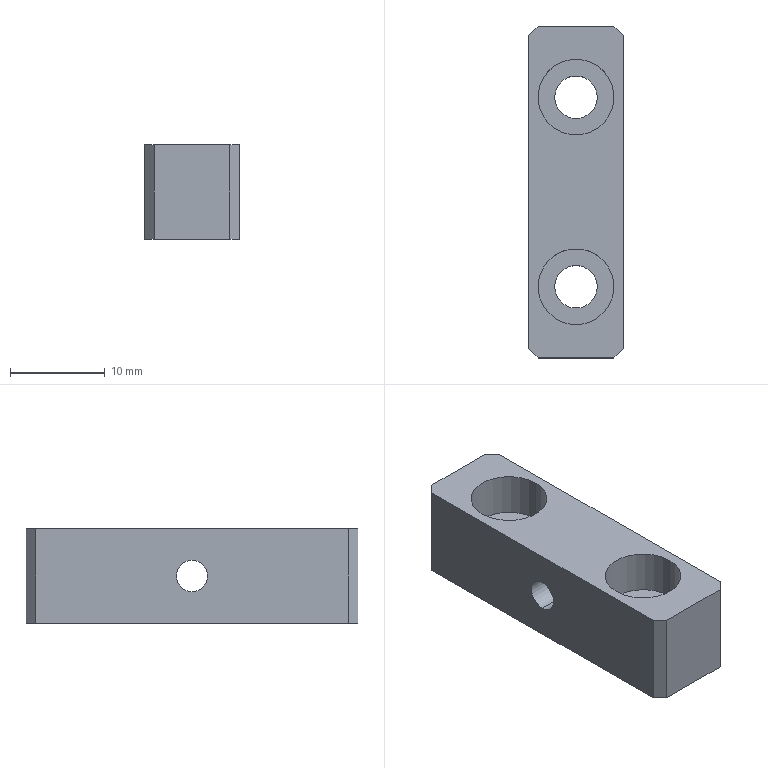Part | STEP file | 08-08 limit block | 1 solid | 22 faces | box 10 x 35 x 10 mm | volume 2760 mm3 | plane 12 | cylinder 10 | commonest cylinder face diameters 4.5 x4 8 x4 3.3 x2
STEP:
#1=CARTESIAN_POINT('',(-5.,0.,6.65));
#2=VERTEX_POINT('',#1);
#3=CARTESIAN_POINT('',(-5.,0.,3.35));
#4=VERTEX_POINT('',#3);
#5=CARTESIAN_POINT('',(-5.,0.,5.));
#6=DIRECTION('',(1.,0.,0.));
#7=DIRECTION('',(0.,0.,-1.));
#8=AXIS2_PLACEMENT_3D('',#5,#6,#7);
#9=CIRCLE('',#8,1.65);
#10=EDGE_CURVE('',#2,#4,#9,.T.);
#11=ORIENTED_EDGE('',*,*,#10,.F.);
#12=CARTESIAN_POINT('',(5.,0.,6.65));
#13=VERTEX_POINT('',#12);
#14=CARTESIAN_POINT('',(5.,0.,6.65));
#15=DIRECTION('',(1.,0.,0.));
#16=VECTOR('',#15,1000.);
#17=LINE('',#14,#16);
#18=EDGE_CURVE('',#2,#13,#17,.T.);
#19=ORIENTED_EDGE('',*,*,#18,.T.);
#20=CARTESIAN_POINT('',(5.,0.,3.35));
#21=VERTEX_POINT('',#20);
#22=CARTESIAN_POINT('',(5.,0.,5.));
#23=DIRECTION('',(1.,0.,0.));
#24=DIRECTION('',(0.,0.,-1.));
#25=AXIS2_PLACEMENT_3D('',#22,#23,#24);
#26=CIRCLE('',#25,1.65);
#27=EDGE_CURVE('',#13,#21,#26,.T.);
#28=ORIENTED_EDGE('',*,*,#27,.T.);
#29=CARTESIAN_POINT('',(5.,0.,3.35));
#30=DIRECTION('',(1.,0.,0.));
#31=VECTOR('',#30,1000.);
#32=LINE('',#29,#31);
#33=EDGE_CURVE('',#4,#21,#32,.T.);
#34=ORIENTED_EDGE('',*,*,#33,.F.);
#35=EDGE_LOOP('',(#11,#19,#28,#34));
#36=FACE_OUTER_BOUND('',#35,.T.);
#37=CARTESIAN_POINT('',(5.,0.,5.));
#38=DIRECTION('',(1.,0.,0.));
#39=DIRECTION('',(0.,0.,-1.));
#40=AXIS2_PLACEMENT_3D('',#37,#38,#39);
#41=CYLINDRICAL_SURFACE('',#40,1.65);
#42=ADVANCED_FACE('',(#36),#41,.F.);
#43=CARTESIAN_POINT('',(-4.,10.,5.4));
#44=VERTEX_POINT('',#43);
#45=CARTESIAN_POINT('',(4.,10.,5.4));
#46=VERTEX_POINT('',#45);
#47=CARTESIAN_POINT('',(0.,10.,5.4));
#48=DIRECTION('',(0.,0.,1.));
#49=DIRECTION('',(1.,0.,0.));
#50=AXIS2_PLACEMENT_3D('',#47,#48,#49);
#51=CIRCLE('',#50,4.);
#52=EDGE_CURVE('',#44,#46,#51,.T.);
#53=ORIENTED_EDGE('',*,*,#52,.F.);
#54=CARTESIAN_POINT('',(-4.,10.,10.));
#55=VERTEX_POINT('',#54);
#56=CARTESIAN_POINT('',(-4.,10.,10.));
#57=DIRECTION('',(0.,0.,1.));
#58=VECTOR('',#57,1000.);
#59=LINE('',#56,#58);
#60=EDGE_CURVE('',#44,#55,#59,.T.);
#61=ORIENTED_EDGE('',*,*,#60,.T.);
#62=CARTESIAN_POINT('',(4.,10.,10.));
#63=VERTEX_POINT('',#62);
#64=CARTESIAN_POINT('',(0.,10.,10.));
#65=DIRECTION('',(0.,0.,1.));
#66=DIRECTION('',(1.,0.,0.));
#67=AXIS2_PLACEMENT_3D('',#64,#65,#66);
#68=CIRCLE('',#67,4.);
#69=EDGE_CURVE('',#55,#63,#68,.T.);
#70=ORIENTED_EDGE('',*,*,#69,.T.);
#71=CARTESIAN_POINT('',(4.,10.,10.));
#72=DIRECTION('',(0.,0.,1.));
#73=VECTOR('',#72,1000.);
#74=LINE('',#71,#73);
#75=EDGE_CURVE('',#46,#63,#74,.T.);
#76=ORIENTED_EDGE('',*,*,#75,.F.);
#77=EDGE_LOOP('',(#53,#61,#70,#76));
#78=FACE_OUTER_BOUND('',#77,.T.);
#79=CARTESIAN_POINT('',(0.,10.,10.));
#80=DIRECTION('',(0.,0.,1.));
#81=DIRECTION('',(1.,0.,0.));
#82=AXIS2_PLACEMENT_3D('',#79,#80,#81);
#83=CYLINDRICAL_SURFACE('',#82,4.);
#84=ADVANCED_FACE('',(#78),#83,.F.);
#85=CARTESIAN_POINT('',(-2.25,10.,0.));
#86=VERTEX_POINT('',#85);
#87=CARTESIAN_POINT('',(2.25,10.,0.));
#88=VERTEX_POINT('',#87);
#89=CARTESIAN_POINT('',(0.,10.,0.));
#90=DIRECTION('',(0.,0.,1.));
#91=DIRECTION('',(1.,0.,0.));
#92=AXIS2_PLACEMENT_3D('',#89,#90,#91);
#93=CIRCLE('',#92,2.25);
#94=EDGE_CURVE('',#86,#88,#93,.T.);
#95=ORIENTED_EDGE('',*,*,#94,.F.);
#96=CARTESIAN_POINT('',(-2.25,10.,5.4));
#97=VERTEX_POINT('',#96);
#98=CARTESIAN_POINT('',(-2.25,10.,10.));
#99=DIRECTION('',(0.,0.,1.));
#100=VECTOR('',#99,1000.);
#101=LINE('',#98,#100);
#102=EDGE_CURVE('',#86,#97,#101,.T.);
#103=ORIENTED_EDGE('',*,*,#102,.T.);
#104=CARTESIAN_POINT('',(2.25,10.,5.4));
#105=VERTEX_POINT('',#104);
#106=CARTESIAN_POINT('',(0.,10.,5.4));
#107=DIRECTION('',(0.,0.,1.));
#108=DIRECTION('',(1.,0.,0.));
#109=AXIS2_PLACEMENT_3D('',#106,#107,#108);
#110=CIRCLE('',#109,2.25);
#111=EDGE_CURVE('',#97,#105,#110,.T.);
#112=ORIENTED_EDGE('',*,*,#111,.T.);
#113=CARTESIAN_POINT('',(2.25,10.,10.));
#114=DIRECTION('',(0.,0.,1.));
#115=VECTOR('',#114,1000.);
#116=LINE('',#113,#115);
#117=EDGE_CURVE('',#88,#105,#116,.T.);
#118=ORIENTED_EDGE('',*,*,#117,.F.);
#119=EDGE_LOOP('',(#95,#103,#112,#118));
#120=FACE_OUTER_BOUND('',#119,.T.);
#121=CARTESIAN_POINT('',(0.,10.,10.));
#122=DIRECTION('',(0.,0.,1.));
#123=DIRECTION('',(1.,0.,0.));
#124=AXIS2_PLACEMENT_3D('',#121,#122,#123);
#125=CYLINDRICAL_SURFACE('',#124,2.25);
#126=ADVANCED_FACE('',(#120),#125,.F.);
#127=CARTESIAN_POINT('',(-4.,-10.,5.4));
#128=VERTEX_POINT('',#127);
#129=CARTESIAN_POINT('',(4.,-10.,5.4));
#130=VERTEX_POINT('',#129);
#131=CARTESIAN_POINT('',(0.,-10.,5.4));
#132=DIRECTION('',(0.,0.,1.));
#133=DIRECTION('',(1.,0.,0.));
#134=AXIS2_PLACEMENT_3D('',#131,#132,#133);
#135=CIRCLE('',#134,4.);
#136=EDGE_CURVE('',#128,#130,#135,.T.);
#137=ORIENTED_EDGE('',*,*,#136,.F.);
#138=CARTESIAN_POINT('',(-4.,-10.,10.));
#139=VERTEX_POINT('',#138);
#140=CARTESIAN_POINT('',(-4.,-10.,10.));
#141=DIRECTION('',(0.,0.,1.));
#142=VECTOR('',#141,1000.);
#143=LINE('',#140,#142);
#144=EDGE_CURVE('',#128,#139,#143,.T.);
#145=ORIENTED_EDGE('',*,*,#144,.T.);
#146=CARTESIAN_POINT('',(4.,-10.,10.));
#147=VERTEX_POINT('',#146);
#148=CARTESIAN_POINT('',(0.,-10.,10.));
#149=DIRECTION('',(0.,0.,1.));
#150=DIRECTION('',(1.,0.,0.));
#151=AXIS2_PLACEMENT_3D('',#148,#149,#150);
#152=CIRCLE('',#151,4.);
#153=EDGE_CURVE('',#139,#147,#152,.T.);
#154=ORIENTED_EDGE('',*,*,#153,.T.);
#155=CARTESIAN_POINT('',(4.,-10.,10.));
#156=DIRECTION('',(0.,0.,1.));
#157=VECTOR('',#156,1000.);
#158=LINE('',#155,#157);
#159=EDGE_CURVE('',#130,#147,#158,.T.);
#160=ORIENTED_EDGE('',*,*,#159,.F.);
#161=EDGE_LOOP('',(#137,#145,#154,#160));
#162=FACE_OUTER_BOUND('',#161,.T.);
#163=CARTESIAN_POINT('',(0.,-10.,10.));
#164=DIRECTION('',(0.,0.,1.));
#165=DIRECTION('',(1.,0.,0.));
#166=AXIS2_PLACEMENT_3D('',#163,#164,#165);
#167=CYLINDRICAL_SURFACE('',#166,4.);
#168=ADVANCED_FACE('',(#162),#167,.F.);
#169=CARTESIAN_POINT('',(-2.25,-10.,0.));
#170=VERTEX_POINT('',#169);
#171=CARTESIAN_POINT('',(2.25,-10.,0.));
#172=VERTEX_POINT('',#171);
#173=CARTESIAN_POINT('',(0.,-10.,0.));
#174=DIRECTION('',(0.,0.,1.));
#175=DIRECTION('',(1.,0.,0.));
#176=AXIS2_PLACEMENT_3D('',#173,#174,#175);
#177=CIRCLE('',#176,2.25);
#178=EDGE_CURVE('',#170,#172,#177,.T.);
#179=ORIENTED_EDGE('',*,*,#178,.F.);
#180=CARTESIAN_POINT('',(-2.25,-10.,5.4));
#181=VERTEX_POINT('',#180);
#182=CARTESIAN_POINT('',(-2.25,-10.,10.));
#183=DIRECTION('',(0.,0.,1.));
#184=VECTOR('',#183,1000.);
#185=LINE('',#182,#184);
#186=EDGE_CURVE('',#170,#181,#185,.T.);
#187=ORIENTED_EDGE('',*,*,#186,.T.);
#188=CARTESIAN_POINT('',(2.25,-10.,5.4));
#189=VERTEX_POINT('',#188);
#190=CARTESIAN_POINT('',(0.,-10.,5.4));
#191=DIRECTION('',(0.,0.,1.));
#192=DIRECTION('',(1.,0.,0.));
#193=AXIS2_PLACEMENT_3D('',#190,#191,#192);
#194=CIRCLE('',#193,2.25);
#195=EDGE_CURVE('',#181,#189,#194,.T.);
#196=ORIENTED_EDGE('',*,*,#195,.T.);
#197=CARTESIAN_POINT('',(2.25,-10.,10.));
#198=DIRECTION('',(0.,0.,1.));
#199=VECTOR('',#198,1000.);
#200=LINE('',#197,#199);
#201=EDGE_CURVE('',#172,#189,#200,.T.);
#202=ORIENTED_EDGE('',*,*,#201,.F.);
#203=EDGE_LOOP('',(#179,#187,#196,#202));
#204=FACE_OUTER_BOUND('',#203,.T.);
#205=CARTESIAN_POINT('',(0.,-10.,10.));
#206=DIRECTION('',(0.,0.,1.));
#207=DIRECTION('',(1.,0.,0.));
#208=AXIS2_PLACEMENT_3D('',#205,#206,#207);
#209=CYLINDRICAL_SURFACE('',#208,2.25);
#210=ADVANCED_FACE('',(#204),#209,.F.);
#211=CARTESIAN_POINT('',(5.,0.,5.));
#212=DIRECTION('',(1.,0.,0.));
#213=DIRECTION('',(0.,0.,-1.));
#214=AXIS2_PLACEMENT_3D('',#211,#212,#213);
#215=CIRCLE('',#214,1.65);
#216=EDGE_CURVE('',#21,#13,#215,.T.);
#217=ORIENTED_EDGE('',*,*,#216,.F.);
#218=ORIENTED_EDGE('',*,*,#27,.F.);
#219=EDGE_LOOP('',(#217,#218));
#220=FACE_BOUND('',#219,.T.);
#221=CARTESIAN_POINT('',(5.,-16.5,10.));
#222=VERTEX_POINT('',#221);
#223=CARTESIAN_POINT('',(5.,16.5,10.));
#224=VERTEX_POINT('',#223);
#225=CARTESIAN_POINT('',(5.,17.5,10.));
#226=DIRECTION('',(0.,1.,0.));
#227=VECTOR('',#226,1000.);
#228=LINE('',#225,#227);
#229=EDGE_CURVE('',#222,#224,#228,.T.);
#230=ORIENTED_EDGE('',*,*,#229,.F.);
#231=CARTESIAN_POINT('',(5.,-16.5,0.));
#232=VERTEX_POINT('',#231);
#233=CARTESIAN_POINT('',(5.,-16.5,10.));
#234=DIRECTION('',(0.,0.,-1.));
#235=VECTOR('',#234,1000.);
#236=LINE('',#233,#235);
#237=EDGE_CURVE('',#222,#232,#236,.T.);
#238=ORIENTED_EDGE('',*,*,#237,.T.);
#239=CARTESIAN_POINT('',(5.,16.5,0.));
#240=VERTEX_POINT('',#239);
#241=CARTESIAN_POINT('',(5.,17.5,0.));
#242=DIRECTION('',(0.,1.,0.));
#243=VECTOR('',#242,1000.);
#244=LINE('',#241,#243);
#245=EDGE_CURVE('',#232,#240,#244,.T.);
#246=ORIENTED_EDGE('',*,*,#245,.T.);
#247=CARTESIAN_POINT('',(5.,16.5,10.));
#248=DIRECTION('',(0.,0.,1.));
#249=VECTOR('',#248,1000.);
#250=LINE('',#247,#249);
#251=EDGE_CURVE('',#240,#224,#250,.T.);
#252=ORIENTED_EDGE('',*,*,#251,.T.);
#253=EDGE_LOOP('',(#230,#238,#246,#252));
#254=FACE_OUTER_BOUND('',#253,.T.);
#255=CARTESIAN_POINT('',(5.,17.5,10.));
#256=DIRECTION('',(-1.,0.,0.));
#257=DIRECTION('',(0.,-1.,0.));
#258=AXIS2_PLACEMENT_3D('',#255,#256,#257);
#259=PLANE('',#258);
#260=ADVANCED_FACE('',(#220,#254),#259,.F.);
#261=CARTESIAN_POINT('',(4.,17.5,10.));
#262=VERTEX_POINT('',#261);
#263=CARTESIAN_POINT('',(-4.,17.5,10.));
#264=VERTEX_POINT('',#263);
#265=CARTESIAN_POINT('',(-5.,17.5,10.));
#266=DIRECTION('',(-1.,0.,0.));
#267=VECTOR('',#266,1000.);
#268=LINE('',#265,#267);
#269=EDGE_CURVE('',#262,#264,#268,.T.);
#270=ORIENTED_EDGE('',*,*,#269,.F.);
#271=CARTESIAN_POINT('',(4.,17.5,0.));
#272=VERTEX_POINT('',#271);
#273=CARTESIAN_POINT('',(4.,17.5,10.));
#274=DIRECTION('',(0.,0.,-1.));
#275=VECTOR('',#274,1000.);
#276=LINE('',#273,#275);
#277=EDGE_CURVE('',#262,#272,#276,.T.);
#278=ORIENTED_EDGE('',*,*,#277,.T.);
#279=CARTESIAN_POINT('',(-4.,17.5,0.));
#280=VERTEX_POINT('',#279);
#281=CARTESIAN_POINT('',(-5.,17.5,0.));
#282=DIRECTION('',(-1.,0.,0.));
#283=VECTOR('',#282,1000.);
#284=LINE('',#281,#283);
#285=EDGE_CURVE('',#272,#280,#284,.T.);
#286=ORIENTED_EDGE('',*,*,#285,.T.);
#287=CARTESIAN_POINT('',(-4.,17.5,10.));
#288=DIRECTION('',(0.,0.,1.));
#289=VECTOR('',#288,1000.);
#290=LINE('',#287,#289);
#291=EDGE_CURVE('',#280,#264,#290,.T.);
#292=ORIENTED_EDGE('',*,*,#291,.T.);
#293=EDGE_LOOP('',(#270,#278,#286,#292));
#294=FACE_OUTER_BOUND('',#293,.T.);
#295=CARTESIAN_POINT('',(-5.,17.5,10.));
#296=DIRECTION('',(0.,-1.,0.));
#297=DIRECTION('',(0.,0.,-1.));
#298=AXIS2_PLACEMENT_3D('',#295,#296,#297);
#299=PLANE('',#298);
#300=ADVANCED_FACE('',(#294),#299,.F.);
#301=CARTESIAN_POINT('',(-5.,0.,5.));
#302=DIRECTION('',(1.,0.,0.));
#303=DIRECTION('',(0.,0.,-1.));
#304=AXIS2_PLACEMENT_3D('',#301,#302,#303);
#305=CIRCLE('',#304,1.65);
#306=EDGE_CURVE('',#4,#2,#305,.T.);
#307=ORIENTED_EDGE('',*,*,#306,.T.);
#308=ORIENTED_EDGE('',*,*,#10,.T.);
#309=EDGE_LOOP('',(#307,#308));
#310=FACE_BOUND('',#309,.T.);
#311=CARTESIAN_POINT('',(-5.,16.5,0.));
#312=VERTEX_POINT('',#311);
#313=CARTESIAN_POINT('',(-5.,-16.5,0.));
#314=VERTEX_POINT('',#313);
#315=CARTESIAN_POINT('',(-5.,17.5,0.));
#316=DIRECTION('',(0.,-1.,0.));
#317=VECTOR('',#316,1000.);
#318=LINE('',#315,#317);
#319=EDGE_CURVE('',#312,#314,#318,.T.);
#320=ORIENTED_EDGE('',*,*,#319,.T.);
#321=CARTESIAN_POINT('',(-5.,-16.5,10.));
#322=VERTEX_POINT('',#321);
#323=CARTESIAN_POINT('',(-5.,-16.5,10.));
#324=DIRECTION('',(0.,0.,1.));
#325=VECTOR('',#324,1000.);
#326=LINE('',#323,#325);
#327=EDGE_CURVE('',#314,#322,#326,.T.);
#328=ORIENTED_EDGE('',*,*,#327,.T.);
#329=CARTESIAN_POINT('',(-5.,16.5,10.));
#330=VERTEX_POINT('',#329);
#331=CARTESIAN_POINT('',(-5.,17.5,10.));
#332=DIRECTION('',(0.,-1.,0.));
#333=VECTOR('',#332,1000.);
#334=LINE('',#331,#333);
#335=EDGE_CURVE('',#330,#322,#334,.T.);
#336=ORIENTED_EDGE('',*,*,#335,.F.);
#337=CARTESIAN_POINT('',(-5.,16.5,10.));
#338=DIRECTION('',(0.,0.,-1.));
#339=VECTOR('',#338,1000.);
#340=LINE('',#337,#339);
#341=EDGE_CURVE('',#330,#312,#340,.T.);
#342=ORIENTED_EDGE('',*,*,#341,.T.);
#343=EDGE_LOOP('',(#320,#328,#336,#342));
#344=FACE_OUTER_BOUND('',#343,.T.);
#345=CARTESIAN_POINT('',(-5.,17.5,10.));
#346=DIRECTION('',(1.,0.,0.));
#347=DIRECTION('',(0.,1.,0.));
#348=AXIS2_PLACEMENT_3D('',#345,#346,#347);
#349=PLANE('',#348);
#350=ADVANCED_FACE('',(#310,#344),#349,.F.);
#351=CARTESIAN_POINT('',(-4.,-17.5,0.));
#352=VERTEX_POINT('',#351);
#353=CARTESIAN_POINT('',(4.,-17.5,0.));
#354=VERTEX_POINT('',#353);
#355=CARTESIAN_POINT('',(-5.,-17.5,0.));
#356=DIRECTION('',(1.,0.,0.));
#357=VECTOR('',#356,1000.);
#358=LINE('',#355,#357);
#359=EDGE_CURVE('',#352,#354,#358,.T.);
#360=ORIENTED_EDGE('',*,*,#359,.T.);
#361=CARTESIAN_POINT('',(4.,-17.5,10.));
#362=VERTEX_POINT('',#361);
#363=CARTESIAN_POINT('',(4.,-17.5,10.));
#364=DIRECTION('',(0.,0.,1.));
#365=VECTOR('',#364,1000.);
#366=LINE('',#363,#365);
#367=EDGE_CURVE('',#354,#362,#366,.T.);
#368=ORIENTED_EDGE('',*,*,#367,.T.);
#369=CARTESIAN_POINT('',(-4.,-17.5,10.));
#370=VERTEX_POINT('',#369);
#371=CARTESIAN_POINT('',(-5.,-17.5,10.));
#372=DIRECTION('',(1.,0.,0.));
#373=VECTOR('',#372,1000.);
#374=LINE('',#371,#373);
#375=EDGE_CURVE('',#370,#362,#374,.T.);
#376=ORIENTED_EDGE('',*,*,#375,.F.);
#377=CARTESIAN_POINT('',(-4.,-17.5,10.));
#378=DIRECTION('',(0.,0.,-1.));
#379=VECTOR('',#378,1000.);
#380=LINE('',#377,#379);
#381=EDGE_CURVE('',#370,#352,#380,.T.);
#382=ORIENTED_EDGE('',*,*,#381,.T.);
#383=EDGE_LOOP('',(#360,#368,#376,#382));
#384=FACE_OUTER_BOUND('',#383,.T.);
#385=CARTESIAN_POINT('',(-5.,-17.5,10.));
#386=DIRECTION('',(0.,1.,0.));
#387=DIRECTION('',(0.,0.,1.));
#388=AXIS2_PLACEMENT_3D('',#385,#386,#387);
#389=PLANE('',#388);
#390=ADVANCED_FACE('',(#384),#389,.F.);
#391=CARTESIAN_POINT('',(0.,10.,10.));
#392=DIRECTION('',(0.,0.,1.));
#393=DIRECTION('',(1.,0.,0.));
#394=AXIS2_PLACEMENT_3D('',#391,#392,#393);
#395=CIRCLE('',#394,4.);
#396=EDGE_CURVE('',#63,#55,#395,.T.);
#397=ORIENTED_EDGE('',*,*,#396,.F.);
#398=ORIENTED_EDGE('',*,*,#69,.F.);
#399=EDGE_LOOP('',(#397,#398));
#400=FACE_BOUND('',#399,.T.);
#401=CARTESIAN_POINT('',(0.,-10.,10.));
#402=DIRECTION('',(0.,0.,1.));
#403=DIRECTION('',(1.,0.,0.));
#404=AXIS2_PLACEMENT_3D('',#401,#402,#403);
#405=CIRCLE('',#404,4.);
#406=EDGE_CURVE('',#147,#139,#405,.T.);
#407=ORIENTED_EDGE('',*,*,#406,.F.);
#408=ORIENTED_EDGE('',*,*,#153,.F.);
#409=EDGE_LOOP('',(#407,#408));
#410=FACE_BOUND('',#409,.T.);
#411=ORIENTED_EDGE('',*,*,#375,.T.);
#412=CARTESIAN_POINT('',(4.5,-17.,10.));
#413=DIRECTION('',(0.7071,0.7071,0.));
#414=VECTOR('',#413,1000.);
#415=LINE('',#412,#414);
#416=EDGE_CURVE('',#362,#222,#415,.T.);
#417=ORIENTED_EDGE('',*,*,#416,.T.);
#418=ORIENTED_EDGE('',*,*,#229,.T.);
#419=CARTESIAN_POINT('',(22.,-0.5,10.));
#420=DIRECTION('',(-0.7071,0.7071,0.));
#421=VECTOR('',#420,1000.);
#422=LINE('',#419,#421);
#423=EDGE_CURVE('',#224,#262,#422,.T.);
#424=ORIENTED_EDGE('',*,*,#423,.T.);
#425=ORIENTED_EDGE('',*,*,#269,.T.);
#426=CARTESIAN_POINT('',(-17.,4.5,10.));
#427=DIRECTION('',(-0.7071,-0.7071,0.));
#428=VECTOR('',#427,1000.);
#429=LINE('',#426,#428);
#430=EDGE_CURVE('',#264,#330,#429,.T.);
#431=ORIENTED_EDGE('',*,*,#430,.T.);
#432=ORIENTED_EDGE('',*,*,#335,.T.);
#433=CARTESIAN_POINT('',(0.5,-22.,10.));
#434=DIRECTION('',(0.7071,-0.7071,0.));
#435=VECTOR('',#434,1000.);
#436=LINE('',#433,#435);
#437=EDGE_CURVE('',#322,#370,#436,.T.);
#438=ORIENTED_EDGE('',*,*,#437,.T.);
#439=EDGE_LOOP('',(#411,#417,#418,#424,#425,#431,#432,#438));
#440=FACE_OUTER_BOUND('',#439,.T.);
#441=CARTESIAN_POINT('',(5.,-17.5,10.));
#442=DIRECTION('',(0.,0.,1.));
#443=DIRECTION('',(1.,0.,0.));
#444=AXIS2_PLACEMENT_3D('',#441,#442,#443);
#445=PLANE('',#444);
#446=ADVANCED_FACE('',(#400,#410,#440),#445,.T.);
#447=CARTESIAN_POINT('',(0.,10.,0.));
#448=DIRECTION('',(0.,0.,1.));
#449=DIRECTION('',(1.,0.,0.));
#450=AXIS2_PLACEMENT_3D('',#447,#448,#449);
#451=CIRCLE('',#450,2.25);
#452=EDGE_CURVE('',#88,#86,#451,.T.);
#453=ORIENTED_EDGE('',*,*,#452,.T.);
#454=ORIENTED_EDGE('',*,*,#94,.T.);
#455=EDGE_LOOP('',(#453,#454));
#456=FACE_BOUND('',#455,.T.);
#457=CARTESIAN_POINT('',(0.,-10.,0.));
#458=DIRECTION('',(0.,0.,1.));
#459=DIRECTION('',(1.,0.,0.));
#460=AXIS2_PLACEMENT_3D('',#457,#458,#459);
#461=CIRCLE('',#460,2.25);
#462=EDGE_CURVE('',#172,#170,#461,.T.);
#463=ORIENTED_EDGE('',*,*,#462,.T.);
#464=ORIENTED_EDGE('',*,*,#178,.T.);
#465=EDGE_LOOP('',(#463,#464));
#466=FACE_BOUND('',#465,.T.);
#467=ORIENTED_EDGE('',*,*,#245,.F.);
#468=CARTESIAN_POINT('',(5.,-16.5,0.));
#469=DIRECTION('',(-0.7071,-0.7071,0.));
#470=VECTOR('',#469,1000.);
#471=LINE('',#468,#470);
#472=EDGE_CURVE('',#232,#354,#471,.T.);
#473=ORIENTED_EDGE('',*,*,#472,.T.);
#474=ORIENTED_EDGE('',*,*,#359,.F.);
#475=CARTESIAN_POINT('',(-4.,-17.5,0.));
#476=DIRECTION('',(-0.7071,0.7071,0.));
#477=VECTOR('',#476,1000.);
#478=LINE('',#475,#477);
#479=EDGE_CURVE('',#352,#314,#478,.T.);
#480=ORIENTED_EDGE('',*,*,#479,.T.);
#481=ORIENTED_EDGE('',*,*,#319,.F.);
#482=CARTESIAN_POINT('',(-5.,16.5,0.));
#483=DIRECTION('',(0.7071,0.7071,0.));
#484=VECTOR('',#483,1000.);
#485=LINE('',#482,#484);
#486=EDGE_CURVE('',#312,#280,#485,.T.);
#487=ORIENTED_EDGE('',*,*,#486,.T.);
#488=ORIENTED_EDGE('',*,*,#285,.F.);
#489=CARTESIAN_POINT('',(4.,17.5,0.));
#490=DIRECTION('',(0.7071,-0.7071,0.));
#491=VECTOR('',#490,1000.);
#492=LINE('',#489,#491);
#493=EDGE_CURVE('',#272,#240,#492,.T.);
#494=ORIENTED_EDGE('',*,*,#493,.T.);
#495=EDGE_LOOP('',(#467,#473,#474,#480,#481,#487,#488,#494));
#496=FACE_OUTER_BOUND('',#495,.T.);
#497=CARTESIAN_POINT('',(5.,-17.5,0.));
#498=DIRECTION('',(0.,0.,1.));
#499=DIRECTION('',(1.,0.,0.));
#500=AXIS2_PLACEMENT_3D('',#497,#498,#499);
#501=PLANE('',#500);
#502=ADVANCED_FACE('',(#456,#466,#496),#501,.F.);
#503=ORIENTED_EDGE('',*,*,#186,.F.);
#504=ORIENTED_EDGE('',*,*,#462,.F.);
#505=ORIENTED_EDGE('',*,*,#201,.T.);
#506=CARTESIAN_POINT('',(0.,-10.,5.4));
#507=DIRECTION('',(0.,0.,1.));
#508=DIRECTION('',(1.,0.,0.));
#509=AXIS2_PLACEMENT_3D('',#506,#507,#508);
#510=CIRCLE('',#509,2.25);
#511=EDGE_CURVE('',#189,#181,#510,.T.);
#512=ORIENTED_EDGE('',*,*,#511,.T.);
#513=EDGE_LOOP('',(#503,#504,#505,#512));
#514=FACE_OUTER_BOUND('',#513,.T.);
#515=CARTESIAN_POINT('',(0.,-10.,10.));
#516=DIRECTION('',(0.,0.,1.));
#517=DIRECTION('',(1.,0.,0.));
#518=AXIS2_PLACEMENT_3D('',#515,#516,#517);
#519=CYLINDRICAL_SURFACE('',#518,2.25);
#520=ADVANCED_FACE('',(#514),#519,.F.);
#521=ORIENTED_EDGE('',*,*,#511,.F.);
#522=ORIENTED_EDGE('',*,*,#195,.F.);
#523=EDGE_LOOP('',(#521,#522));
#524=FACE_BOUND('',#523,.T.);
#525=CARTESIAN_POINT('',(0.,-10.,5.4));
#526=DIRECTION('',(0.,0.,1.));
#527=DIRECTION('',(1.,0.,0.));
#528=AXIS2_PLACEMENT_3D('',#525,#526,#527);
#529=CIRCLE('',#528,4.);
#530=EDGE_CURVE('',#130,#128,#529,.T.);
#531=ORIENTED_EDGE('',*,*,#530,.T.);
#532=ORIENTED_EDGE('',*,*,#136,.T.);
#533=EDGE_LOOP('',(#531,#532));
#534=FACE_OUTER_BOUND('',#533,.T.);
#535=CARTESIAN_POINT('',(2.25,-10.,5.4));
#536=DIRECTION('',(0.,0.,-1.));
#537=DIRECTION('',(-1.,0.,0.));
#538=AXIS2_PLACEMENT_3D('',#535,#536,#537);
#539=PLANE('',#538);
#540=ADVANCED_FACE('',(#524,#534),#539,.F.);
#541=ORIENTED_EDGE('',*,*,#144,.F.);
#542=ORIENTED_EDGE('',*,*,#530,.F.);
#543=ORIENTED_EDGE('',*,*,#159,.T.);
#544=ORIENTED_EDGE('',*,*,#406,.T.);
#545=EDGE_LOOP('',(#541,#542,#543,#544));
#546=FACE_OUTER_BOUND('',#545,.T.);
#547=CARTESIAN_POINT('',(0.,-10.,10.));
#548=DIRECTION('',(0.,0.,1.));
#549=DIRECTION('',(1.,0.,0.));
#550=AXIS2_PLACEMENT_3D('',#547,#548,#549);
#551=CYLINDRICAL_SURFACE('',#550,4.);
#552=ADVANCED_FACE('',(#546),#551,.F.);
#553=ORIENTED_EDGE('',*,*,#102,.F.);
#554=ORIENTED_EDGE('',*,*,#452,.F.);
#555=ORIENTED_EDGE('',*,*,#117,.T.);
#556=CARTESIAN_POINT('',(0.,10.,5.4));
#557=DIRECTION('',(0.,0.,1.));
#558=DIRECTION('',(1.,0.,0.));
#559=AXIS2_PLACEMENT_3D('',#556,#557,#558);
#560=CIRCLE('',#559,2.25);
#561=EDGE_CURVE('',#105,#97,#560,.T.);
#562=ORIENTED_EDGE('',*,*,#561,.T.);
#563=EDGE_LOOP('',(#553,#554,#555,#562));
#564=FACE_OUTER_BOUND('',#563,.T.);
#565=CARTESIAN_POINT('',(0.,10.,10.));
#566=DIRECTION('',(0.,0.,1.));
#567=DIRECTION('',(1.,0.,0.));
#568=AXIS2_PLACEMENT_3D('',#565,#566,#567);
#569=CYLINDRICAL_SURFACE('',#568,2.25);
#570=ADVANCED_FACE('',(#564),#569,.F.);
#571=ORIENTED_EDGE('',*,*,#561,.F.);
#572=ORIENTED_EDGE('',*,*,#111,.F.);
#573=EDGE_LOOP('',(#571,#572));
#574=FACE_BOUND('',#573,.T.);
#575=CARTESIAN_POINT('',(0.,10.,5.4));
#576=DIRECTION('',(0.,0.,1.));
#577=DIRECTION('',(1.,0.,0.));
#578=AXIS2_PLACEMENT_3D('',#575,#576,#577);
#579=CIRCLE('',#578,4.);
#580=EDGE_CURVE('',#46,#44,#579,.T.);
#581=ORIENTED_EDGE('',*,*,#580,.T.);
#582=ORIENTED_EDGE('',*,*,#52,.T.);
#583=EDGE_LOOP('',(#581,#582));
#584=FACE_OUTER_BOUND('',#583,.T.);
#585=CARTESIAN_POINT('',(2.25,10.,5.4));
#586=DIRECTION('',(0.,0.,-1.));
#587=DIRECTION('',(-1.,0.,0.));
#588=AXIS2_PLACEMENT_3D('',#585,#586,#587);
#589=PLANE('',#588);
#590=ADVANCED_FACE('',(#574,#584),#589,.F.);
#591=ORIENTED_EDGE('',*,*,#60,.F.);
#592=ORIENTED_EDGE('',*,*,#580,.F.);
#593=ORIENTED_EDGE('',*,*,#75,.T.);
#594=ORIENTED_EDGE('',*,*,#396,.T.);
#595=EDGE_LOOP('',(#591,#592,#593,#594));
#596=FACE_OUTER_BOUND('',#595,.T.);
#597=CARTESIAN_POINT('',(0.,10.,10.));
#598=DIRECTION('',(0.,0.,1.));
#599=DIRECTION('',(1.,0.,0.));
#600=AXIS2_PLACEMENT_3D('',#597,#598,#599);
#601=CYLINDRICAL_SURFACE('',#600,4.);
#602=ADVANCED_FACE('',(#596),#601,.F.);
#603=ORIENTED_EDGE('',*,*,#416,.F.);
#604=ORIENTED_EDGE('',*,*,#367,.F.);
#605=ORIENTED_EDGE('',*,*,#472,.F.);
#606=ORIENTED_EDGE('',*,*,#237,.F.);
#607=EDGE_LOOP('',(#603,#604,#605,#606));
#608=FACE_OUTER_BOUND('',#607,.T.);
#609=CARTESIAN_POINT('',(5.,-16.5,10.));
#610=DIRECTION('',(-0.7071,0.7071,0.));
#611=DIRECTION('',(-0.7071,-0.7071,0.));
#612=AXIS2_PLACEMENT_3D('',#609,#610,#611);
#613=PLANE('',#612);
#614=ADVANCED_FACE('',(#608),#613,.F.);
#615=ORIENTED_EDGE('',*,*,#437,.F.);
#616=ORIENTED_EDGE('',*,*,#327,.F.);
#617=ORIENTED_EDGE('',*,*,#479,.F.);
#618=ORIENTED_EDGE('',*,*,#381,.F.);
#619=EDGE_LOOP('',(#615,#616,#617,#618));
#620=FACE_OUTER_BOUND('',#619,.T.);
#621=CARTESIAN_POINT('',(-4.,-17.5,10.));
#622=DIRECTION('',(0.7071,0.7071,0.));
#623=DIRECTION('',(-0.7071,0.7071,0.));
#624=AXIS2_PLACEMENT_3D('',#621,#622,#623);
#625=PLANE('',#624);
#626=ADVANCED_FACE('',(#620),#625,.F.);
#627=ORIENTED_EDGE('',*,*,#423,.F.);
#628=ORIENTED_EDGE('',*,*,#251,.F.);
#629=ORIENTED_EDGE('',*,*,#493,.F.);
#630=ORIENTED_EDGE('',*,*,#277,.F.);
#631=EDGE_LOOP('',(#627,#628,#629,#630));
#632=FACE_OUTER_BOUND('',#631,.T.);
#633=CARTESIAN_POINT('',(4.,17.5,10.));
#634=DIRECTION('',(-0.7071,-0.7071,0.));
#635=DIRECTION('',(0.7071,-0.7071,0.));
#636=AXIS2_PLACEMENT_3D('',#633,#634,#635);
#637=PLANE('',#636);
#638=ADVANCED_FACE('',(#632),#637,.F.);
#639=ORIENTED_EDGE('',*,*,#430,.F.);
#640=ORIENTED_EDGE('',*,*,#291,.F.);
#641=ORIENTED_EDGE('',*,*,#486,.F.);
#642=ORIENTED_EDGE('',*,*,#341,.F.);
#643=EDGE_LOOP('',(#639,#640,#641,#642));
#644=FACE_OUTER_BOUND('',#643,.T.);
#645=CARTESIAN_POINT('',(-5.,16.5,10.));
#646=DIRECTION('',(0.7071,-0.7071,0.));
#647=DIRECTION('',(0.7071,0.7071,0.));
#648=AXIS2_PLACEMENT_3D('',#645,#646,#647);
#649=PLANE('',#648);
#650=ADVANCED_FACE('',(#644),#649,.F.);
#651=ORIENTED_EDGE('',*,*,#18,.F.);
#652=ORIENTED_EDGE('',*,*,#306,.F.);
#653=ORIENTED_EDGE('',*,*,#33,.T.);
#654=ORIENTED_EDGE('',*,*,#216,.T.);
#655=EDGE_LOOP('',(#651,#652,#653,#654));
#656=FACE_OUTER_BOUND('',#655,.T.);
#657=CARTESIAN_POINT('',(5.,0.,5.));
#658=DIRECTION('',(1.,0.,0.));
#659=DIRECTION('',(0.,0.,-1.));
#660=AXIS2_PLACEMENT_3D('',#657,#658,#659);
#661=CYLINDRICAL_SURFACE('',#660,1.65);
#662=ADVANCED_FACE('',(#656),#661,.F.);
#663=CLOSED_SHELL('',(#42,#84,#126,#168,#210,#260,#300,#350,#390,#446,#502,#520,#540,#552,#570,#590,#602,#614,#626,#638,#650,#662));
#664=MANIFOLD_SOLID_BREP('',#663);
#665=CARTESIAN_POINT('',(0.,0.,0.));
#666=DIRECTION('',(0.,0.,1.));
#667=DIRECTION('',(1.,0.,0.));
#668=AXIS2_PLACEMENT_3D('',#665,#666,#667);
#669=(LENGTH_UNIT()NAMED_UNIT(*)SI_UNIT(.MILLI.,.METRE.));
#670=UNCERTAINTY_MEASURE_WITH_UNIT(LENGTH_MEASURE(0.00001),#669,'','');
#671=(NAMED_UNIT(*)PLANE_ANGLE_UNIT()SI_UNIT($,.RADIAN.));
#672=(NAMED_UNIT(*)SI_UNIT($,.STERADIAN.)SOLID_ANGLE_UNIT());
#673=(GEOMETRIC_REPRESENTATION_CONTEXT(3)GLOBAL_UNCERTAINTY_ASSIGNED_CONTEXT((#670))GLOBAL_UNIT_ASSIGNED_CONTEXT((#669,#671,#672))REPRESENTATION_CONTEXT('',''));
#674=ADVANCED_BREP_SHAPE_REPRESENTATION('',(#664,#668),#673);